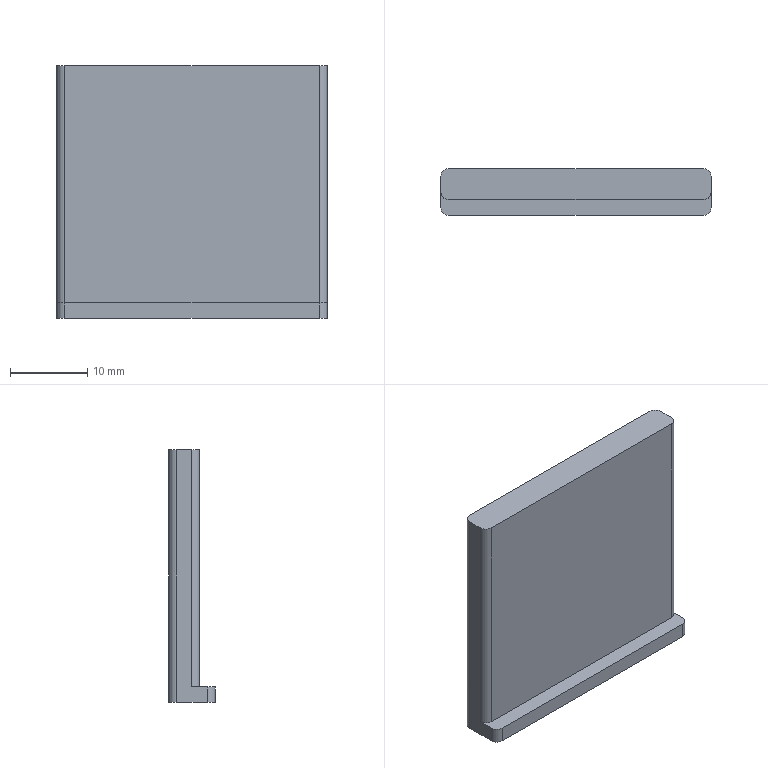Part | STEP file | 1 solid | 14 faces | box 34.97 x 6 x 32.7 mm | volume 4654 mm3 | plane 8 | cylinder 6 | commonest cylinder face diameters 2 x6
STEP:
#1=CARTESIAN_POINT('',(0.,0.,0.));
#2=DIRECTION('',(0.,0.,1.));
#3=DIRECTION('',(1.,0.,0.));
#4=AXIS2_PLACEMENT_3D('',#1,#2,#3);
#5=CARTESIAN_POINT('',(1348.732,487.51,23.619));
#6=VERTEX_POINT('',#5);
#7=CARTESIAN_POINT('',(1315.762,487.51,23.619));
#8=VERTEX_POINT('',#7);
#9=CARTESIAN_POINT('',(1314.747,487.51,23.619));
#10=DIRECTION('',(-1.,0.,0.));
#11=VECTOR('',#10,1.);
#12=LINE('',#9,#11);
#13=CARTESIAN_POINT('',(1314.747,487.51,227.429));
#14=DIRECTION('',(0.,1.,0.));
#15=DIRECTION('',(0.,0.,-1.));
#16=AXIS2_PLACEMENT_3D('',#13,#14,#15);
#17=PLANE('',#16);
#18=CARTESIAN_POINT('',(203.81,0.));
#19=DIRECTION('',(0.,1.));
#20=VECTOR('',#19,1.);
#21=LINE('',#18,#20);
#22=(GEOMETRIC_REPRESENTATION_CONTEXT(2)PARAMETRIC_REPRESENTATION_CONTEXT()REPRESENTATION_CONTEXT('',''));
#23=DEFINITIONAL_REPRESENTATION('',(#21),#22);
#24=PCURVE('',#17,#23);
#25=CARTESIAN_POINT('',(1317.247,584.995,23.619));
#26=DIRECTION('',(0.,0.,-1.));
#27=DIRECTION('',(-1.,0.,0.));
#28=AXIS2_PLACEMENT_3D('',#25,#26,#27);
#29=PLANE('',#28);
#30=CARTESIAN_POINT('',(2.5,-97.485));
#31=DIRECTION('',(1.,0.));
#32=VECTOR('',#31,1.);
#33=LINE('',#30,#32);
#34=(GEOMETRIC_REPRESENTATION_CONTEXT(2)PARAMETRIC_REPRESENTATION_CONTEXT()REPRESENTATION_CONTEXT('',''));
#35=DEFINITIONAL_REPRESENTATION('',(#33),#34);
#36=PCURVE('',#29,#35);
#37=SURFACE_CURVE('',#12,(#24,#36),.PCURVE_S1.);
#38=EDGE_CURVE('',#6,#8,#37,.T.);
#39=ORIENTED_EDGE('',*,*,#38,.T.);
#40=CARTESIAN_POINT('',(1315.762,487.51,-7.081));
#41=VERTEX_POINT('',#40);
#42=CARTESIAN_POINT('',(1315.762,487.51,227.429));
#43=DIRECTION('',(0.,0.,-1.));
#44=VECTOR('',#43,1.);
#45=LINE('',#42,#44);
#46=CARTESIAN_POINT('',(0.,-1.015));
#47=DIRECTION('',(1.,0.));
#48=VECTOR('',#47,1.);
#49=LINE('',#46,#48);
#50=(GEOMETRIC_REPRESENTATION_CONTEXT(2)PARAMETRIC_REPRESENTATION_CONTEXT()REPRESENTATION_CONTEXT('',''));
#51=DEFINITIONAL_REPRESENTATION('',(#49),#50);
#52=PCURVE('',#17,#51);
#53=CARTESIAN_POINT('',(1315.762,488.51,227.429));
#54=DIRECTION('',(0.,0.,-1.));
#55=DIRECTION('',(-1.,0.,0.));
#56=AXIS2_PLACEMENT_3D('',#53,#54,#55);
#57=CYLINDRICAL_SURFACE('',#56,1.);
#58=CARTESIAN_POINT('',(4.712,0.));
#59=DIRECTION('',(0.,1.));
#60=VECTOR('',#59,1.);
#61=LINE('',#58,#60);
#62=(GEOMETRIC_REPRESENTATION_CONTEXT(2)PARAMETRIC_REPRESENTATION_CONTEXT()REPRESENTATION_CONTEXT('',''));
#63=DEFINITIONAL_REPRESENTATION('',(#61),#62);
#64=PCURVE('',#57,#63);
#65=SURFACE_CURVE('',#45,(#52,#64),.PCURVE_S1.);
#66=EDGE_CURVE('',#8,#41,#65,.T.);
#67=ORIENTED_EDGE('',*,*,#66,.T.);
#68=CARTESIAN_POINT('',(1348.732,487.51,-7.081));
#69=VERTEX_POINT('',#68);
#70=CARTESIAN_POINT('',(1349.732,487.51,-7.081));
#71=DIRECTION('',(-1.,0.,0.));
#72=VECTOR('',#71,1.);
#73=LINE('',#70,#72);
#74=CARTESIAN_POINT('',(234.51,-34.985));
#75=DIRECTION('',(0.,1.));
#76=VECTOR('',#75,1.);
#77=LINE('',#74,#76);
#78=(GEOMETRIC_REPRESENTATION_CONTEXT(2)PARAMETRIC_REPRESENTATION_CONTEXT()REPRESENTATION_CONTEXT('',''));
#79=DEFINITIONAL_REPRESENTATION('',(#77),#78);
#80=PCURVE('',#17,#79);
#81=CARTESIAN_POINT('',(1349.732,487.51,-7.081));
#82=DIRECTION('',(0.,0.,1.));
#83=DIRECTION('',(1.,0.,0.));
#84=AXIS2_PLACEMENT_3D('',#81,#82,#83);
#85=PLANE('',#84);
#86=CARTESIAN_POINT('',(0.,0.));
#87=DIRECTION('',(-1.,0.));
#88=VECTOR('',#87,1.);
#89=LINE('',#86,#88);
#90=(GEOMETRIC_REPRESENTATION_CONTEXT(2)PARAMETRIC_REPRESENTATION_CONTEXT()REPRESENTATION_CONTEXT('',''));
#91=DEFINITIONAL_REPRESENTATION('',(#89),#90);
#92=PCURVE('',#85,#91);
#93=SURFACE_CURVE('',#73,(#80,#92),.PCURVE_S1.);
#94=EDGE_CURVE('',#69,#41,#93,.T.);
#95=ORIENTED_EDGE('',*,*,#94,.F.);
#96=CARTESIAN_POINT('',(1348.732,487.51,227.429));
#97=DIRECTION('',(0.,0.,1.));
#98=VECTOR('',#97,1.);
#99=LINE('',#96,#98);
#100=CARTESIAN_POINT('',(0.,-33.985));
#101=DIRECTION('',(-1.,0.));
#102=VECTOR('',#101,1.);
#103=LINE('',#100,#102);
#104=(GEOMETRIC_REPRESENTATION_CONTEXT(2)PARAMETRIC_REPRESENTATION_CONTEXT()REPRESENTATION_CONTEXT('',''));
#105=DEFINITIONAL_REPRESENTATION('',(#103),#104);
#106=PCURVE('',#17,#105);
#107=CARTESIAN_POINT('',(1348.732,488.51,227.429));
#108=DIRECTION('',(0.,0.,-1.));
#109=DIRECTION('',(-1.,0.,0.));
#110=AXIS2_PLACEMENT_3D('',#107,#108,#109);
#111=CYLINDRICAL_SURFACE('',#110,1.);
#112=CARTESIAN_POINT('',(4.712,0.));
#113=DIRECTION('',(0.,-1.));
#114=VECTOR('',#113,1.);
#115=LINE('',#112,#114);
#116=(GEOMETRIC_REPRESENTATION_CONTEXT(2)PARAMETRIC_REPRESENTATION_CONTEXT()REPRESENTATION_CONTEXT('',''));
#117=DEFINITIONAL_REPRESENTATION('',(#115),#116);
#118=PCURVE('',#111,#117);
#119=SURFACE_CURVE('',#99,(#106,#118),.PCURVE_S1.);
#120=EDGE_CURVE('',#69,#6,#119,.T.);
#121=ORIENTED_EDGE('',*,*,#120,.T.);
#122=EDGE_LOOP('',(#39,#67,#95,#121));
#123=FACE_BOUND('',#122,.T.);
#124=ADVANCED_FACE('',(#123),#17,.F.);
#125=CARTESIAN_POINT('',(1314.762,488.51,23.619));
#126=VERTEX_POINT('',#125);
#127=CARTESIAN_POINT('',(1314.762,490.48,23.619));
#128=VERTEX_POINT('',#127);
#129=CARTESIAN_POINT('',(1314.762,491.495,23.619));
#130=DIRECTION('',(0.,1.,0.));
#131=VECTOR('',#130,1.);
#132=LINE('',#129,#131);
#133=CARTESIAN_POINT('',(2.485,-93.5));
#134=DIRECTION('',(0.,1.));
#135=VECTOR('',#134,1.);
#136=LINE('',#133,#135);
#137=(GEOMETRIC_REPRESENTATION_CONTEXT(2)PARAMETRIC_REPRESENTATION_CONTEXT()REPRESENTATION_CONTEXT('',''));
#138=DEFINITIONAL_REPRESENTATION('',(#136),#137);
#139=PCURVE('',#29,#138);
#140=CARTESIAN_POINT('',(1314.762,491.495,227.429));
#141=DIRECTION('',(1.,0.,0.));
#142=DIRECTION('',(0.,0.,-1.));
#143=AXIS2_PLACEMENT_3D('',#140,#141,#142);
#144=PLANE('',#143);
#145=CARTESIAN_POINT('',(203.81,0.));
#146=DIRECTION('',(0.,1.));
#147=VECTOR('',#146,1.);
#148=LINE('',#145,#147);
#149=(GEOMETRIC_REPRESENTATION_CONTEXT(2)PARAMETRIC_REPRESENTATION_CONTEXT()REPRESENTATION_CONTEXT('',''));
#150=DEFINITIONAL_REPRESENTATION('',(#148),#149);
#151=PCURVE('',#144,#150);
#152=SURFACE_CURVE('',#132,(#139,#151),.PCURVE_S1.);
#153=EDGE_CURVE('',#126,#128,#152,.T.);
#154=ORIENTED_EDGE('',*,*,#153,.F.);
#155=CARTESIAN_POINT('',(1315.762,488.51,23.619));
#156=DIRECTION('',(0.,0.,1.));
#157=DIRECTION('',(1.,0.,0.));
#158=AXIS2_PLACEMENT_3D('',#155,#156,#157);
#159=CIRCLE('',#158,1.);
#160=CARTESIAN_POINT('',(0.4851,-96.485));
#161=CARTESIAN_POINT('',(0.4851,-94.753));
#162=CARTESIAN_POINT('',(1.985,-95.619));
#163=CARTESIAN_POINT('',(3.485,-96.485));
#164=CARTESIAN_POINT('',(1.985,-97.351));
#165=CARTESIAN_POINT('',(0.4851,-98.217));
#166=CARTESIAN_POINT('',(0.4851,-96.485));
#167=(BOUNDED_CURVE()B_SPLINE_CURVE(2,(#160,#161,#162,#163,#164,#165,#166),.UNSPECIFIED.,.T.,.F.)B_SPLINE_CURVE_WITH_KNOTS((1,2,2,2,2,1),(-2.094,0.,2.094,4.189,6.283,8.378),.UNSPECIFIED.)CURVE()GEOMETRIC_REPRESENTATION_ITEM()RATIONAL_B_SPLINE_CURVE((1.,0.5,1.,0.5,1.,0.5,1.))REPRESENTATION_ITEM(''));
#168=(GEOMETRIC_REPRESENTATION_CONTEXT(2)PARAMETRIC_REPRESENTATION_CONTEXT()REPRESENTATION_CONTEXT('',''));
#169=DEFINITIONAL_REPRESENTATION('',(#167),#168);
#170=PCURVE('',#29,#169);
#171=CARTESIAN_POINT('',(9.425,203.81));
#172=DIRECTION('',(-1.,0.));
#173=VECTOR('',#172,1.);
#174=LINE('',#171,#173);
#175=(GEOMETRIC_REPRESENTATION_CONTEXT(2)PARAMETRIC_REPRESENTATION_CONTEXT()REPRESENTATION_CONTEXT('',''));
#176=DEFINITIONAL_REPRESENTATION('',(#174),#175);
#177=PCURVE('',#57,#176);
#178=SURFACE_CURVE('',#159,(#170,#177),.PCURVE_S1.);
#179=EDGE_CURVE('',#126,#8,#178,.T.);
#180=ORIENTED_EDGE('',*,*,#179,.T.);
#181=ORIENTED_EDGE('',*,*,#38,.F.);
#182=CARTESIAN_POINT('',(1349.732,488.51,23.619));
#183=VERTEX_POINT('',#182);
#184=CARTESIAN_POINT('',(1348.732,488.51,23.619));
#185=DIRECTION('',(0.,0.,1.));
#186=DIRECTION('',(1.,0.,0.));
#187=AXIS2_PLACEMENT_3D('',#184,#185,#186);
#188=CIRCLE('',#187,1.);
#189=CARTESIAN_POINT('',(-32.485,-96.485));
#190=CARTESIAN_POINT('',(-32.485,-94.753));
#191=CARTESIAN_POINT('',(-30.985,-95.619));
#192=CARTESIAN_POINT('',(-29.485,-96.485));
#193=CARTESIAN_POINT('',(-30.985,-97.351));
#194=CARTESIAN_POINT('',(-32.485,-98.217));
#195=CARTESIAN_POINT('',(-32.485,-96.485));
#196=(BOUNDED_CURVE()B_SPLINE_CURVE(2,(#189,#190,#191,#192,#193,#194,#195),.UNSPECIFIED.,.T.,.F.)B_SPLINE_CURVE_WITH_KNOTS((1,2,2,2,2,1),(-2.094,0.,2.094,4.189,6.283,8.378),.UNSPECIFIED.)CURVE()GEOMETRIC_REPRESENTATION_ITEM()RATIONAL_B_SPLINE_CURVE((1.,0.5,1.,0.5,1.,0.5,1.))REPRESENTATION_ITEM(''));
#197=(GEOMETRIC_REPRESENTATION_CONTEXT(2)PARAMETRIC_REPRESENTATION_CONTEXT()REPRESENTATION_CONTEXT('',''));
#198=DEFINITIONAL_REPRESENTATION('',(#196),#197);
#199=PCURVE('',#29,#198);
#200=CARTESIAN_POINT('',(9.425,203.81));
#201=DIRECTION('',(-1.,0.));
#202=VECTOR('',#201,1.);
#203=LINE('',#200,#202);
#204=(GEOMETRIC_REPRESENTATION_CONTEXT(2)PARAMETRIC_REPRESENTATION_CONTEXT()REPRESENTATION_CONTEXT('',''));
#205=DEFINITIONAL_REPRESENTATION('',(#203),#204);
#206=PCURVE('',#111,#205);
#207=SURFACE_CURVE('',#188,(#199,#206),.PCURVE_S1.);
#208=EDGE_CURVE('',#6,#183,#207,.T.);
#209=ORIENTED_EDGE('',*,*,#208,.T.);
#210=CARTESIAN_POINT('',(1349.732,490.48,23.619));
#211=VERTEX_POINT('',#210);
#212=CARTESIAN_POINT('',(1349.732,487.495,23.619));
#213=DIRECTION('',(0.,-1.,0.));
#214=VECTOR('',#213,1.);
#215=LINE('',#212,#214);
#216=CARTESIAN_POINT('',(-32.485,-97.5));
#217=DIRECTION('',(0.,-1.));
#218=VECTOR('',#217,1.);
#219=LINE('',#216,#218);
#220=(GEOMETRIC_REPRESENTATION_CONTEXT(2)PARAMETRIC_REPRESENTATION_CONTEXT()REPRESENTATION_CONTEXT('',''));
#221=DEFINITIONAL_REPRESENTATION('',(#219),#220);
#222=PCURVE('',#29,#221);
#223=CARTESIAN_POINT('',(1349.732,487.495,227.429));
#224=DIRECTION('',(-1.,0.,0.));
#225=DIRECTION('',(0.,0.,1.));
#226=AXIS2_PLACEMENT_3D('',#223,#224,#225);
#227=PLANE('',#226);
#228=CARTESIAN_POINT('',(-203.81,0.));
#229=DIRECTION('',(0.,-1.));
#230=VECTOR('',#229,1.);
#231=LINE('',#228,#230);
#232=(GEOMETRIC_REPRESENTATION_CONTEXT(2)PARAMETRIC_REPRESENTATION_CONTEXT()REPRESENTATION_CONTEXT('',''));
#233=DEFINITIONAL_REPRESENTATION('',(#231),#232);
#234=PCURVE('',#227,#233);
#235=SURFACE_CURVE('',#215,(#222,#234),.PCURVE_S1.);
#236=EDGE_CURVE('',#211,#183,#235,.T.);
#237=ORIENTED_EDGE('',*,*,#236,.F.);
#238=CARTESIAN_POINT('',(1348.732,491.48,23.619));
#239=VERTEX_POINT('',#238);
#240=CARTESIAN_POINT('',(1348.732,490.48,23.619));
#241=DIRECTION('',(0.,0.,1.));
#242=DIRECTION('',(1.,0.,0.));
#243=AXIS2_PLACEMENT_3D('',#240,#241,#242);
#244=CIRCLE('',#243,1.);
#245=CARTESIAN_POINT('',(-32.485,-94.515));
#246=CARTESIAN_POINT('',(-32.485,-92.783));
#247=CARTESIAN_POINT('',(-30.985,-93.649));
#248=CARTESIAN_POINT('',(-29.485,-94.515));
#249=CARTESIAN_POINT('',(-30.985,-95.381));
#250=CARTESIAN_POINT('',(-32.485,-96.247));
#251=CARTESIAN_POINT('',(-32.485,-94.515));
#252=(BOUNDED_CURVE()B_SPLINE_CURVE(2,(#245,#246,#247,#248,#249,#250,#251),.UNSPECIFIED.,.T.,.F.)B_SPLINE_CURVE_WITH_KNOTS((1,2,2,2,2,1),(-2.094,0.,2.094,4.189,6.283,8.378),.UNSPECIFIED.)CURVE()GEOMETRIC_REPRESENTATION_ITEM()RATIONAL_B_SPLINE_CURVE((1.,0.5,1.,0.5,1.,0.5,1.))REPRESENTATION_ITEM(''));
#253=(GEOMETRIC_REPRESENTATION_CONTEXT(2)PARAMETRIC_REPRESENTATION_CONTEXT()REPRESENTATION_CONTEXT('',''));
#254=DEFINITIONAL_REPRESENTATION('',(#252),#253);
#255=PCURVE('',#29,#254);
#256=CARTESIAN_POINT('',(1348.732,490.48,227.429));
#257=DIRECTION('',(0.,0.,-1.));
#258=DIRECTION('',(-1.,0.,0.));
#259=AXIS2_PLACEMENT_3D('',#256,#257,#258);
#260=CYLINDRICAL_SURFACE('',#259,1.);
#261=CARTESIAN_POINT('',(3.142,203.81));
#262=DIRECTION('',(-1.,0.));
#263=VECTOR('',#262,1.);
#264=LINE('',#261,#263);
#265=(GEOMETRIC_REPRESENTATION_CONTEXT(2)PARAMETRIC_REPRESENTATION_CONTEXT()REPRESENTATION_CONTEXT('',''));
#266=DEFINITIONAL_REPRESENTATION('',(#264),#265);
#267=PCURVE('',#260,#266);
#268=SURFACE_CURVE('',#244,(#255,#267),.PCURVE_S1.);
#269=EDGE_CURVE('',#211,#239,#268,.T.);
#270=ORIENTED_EDGE('',*,*,#269,.T.);
#271=CARTESIAN_POINT('',(1315.762,491.48,23.619));
#272=VERTEX_POINT('',#271);
#273=CARTESIAN_POINT('',(1349.747,491.48,23.619));
#274=DIRECTION('',(1.,0.,0.));
#275=VECTOR('',#274,1.);
#276=LINE('',#273,#275);
#277=CARTESIAN_POINT('',(-32.5,-93.515));
#278=DIRECTION('',(-1.,0.));
#279=VECTOR('',#278,1.);
#280=LINE('',#277,#279);
#281=(GEOMETRIC_REPRESENTATION_CONTEXT(2)PARAMETRIC_REPRESENTATION_CONTEXT()REPRESENTATION_CONTEXT('',''));
#282=DEFINITIONAL_REPRESENTATION('',(#280),#281);
#283=PCURVE('',#29,#282);
#284=CARTESIAN_POINT('',(1349.747,491.48,227.429));
#285=DIRECTION('',(0.,-1.,0.));
#286=DIRECTION('',(0.,0.,1.));
#287=AXIS2_PLACEMENT_3D('',#284,#285,#286);
#288=PLANE('',#287);
#289=CARTESIAN_POINT('',(-203.81,0.));
#290=DIRECTION('',(0.,-1.));
#291=VECTOR('',#290,1.);
#292=LINE('',#289,#291);
#293=(GEOMETRIC_REPRESENTATION_CONTEXT(2)PARAMETRIC_REPRESENTATION_CONTEXT()REPRESENTATION_CONTEXT('',''));
#294=DEFINITIONAL_REPRESENTATION('',(#292),#293);
#295=PCURVE('',#288,#294);
#296=SURFACE_CURVE('',#276,(#283,#295),.PCURVE_S1.);
#297=EDGE_CURVE('',#272,#239,#296,.T.);
#298=ORIENTED_EDGE('',*,*,#297,.F.);
#299=CARTESIAN_POINT('',(1315.762,490.48,23.619));
#300=DIRECTION('',(0.,0.,1.));
#301=DIRECTION('',(1.,0.,0.));
#302=AXIS2_PLACEMENT_3D('',#299,#300,#301);
#303=CIRCLE('',#302,1.);
#304=CARTESIAN_POINT('',(0.4851,-94.515));
#305=CARTESIAN_POINT('',(0.4851,-92.783));
#306=CARTESIAN_POINT('',(1.985,-93.649));
#307=CARTESIAN_POINT('',(3.485,-94.515));
#308=CARTESIAN_POINT('',(1.985,-95.381));
#309=CARTESIAN_POINT('',(0.4851,-96.247));
#310=CARTESIAN_POINT('',(0.4851,-94.515));
#311=(BOUNDED_CURVE()B_SPLINE_CURVE(2,(#304,#305,#306,#307,#308,#309,#310),.UNSPECIFIED.,.T.,.F.)B_SPLINE_CURVE_WITH_KNOTS((1,2,2,2,2,1),(-2.094,0.,2.094,4.189,6.283,8.378),.UNSPECIFIED.)CURVE()GEOMETRIC_REPRESENTATION_ITEM()RATIONAL_B_SPLINE_CURVE((1.,0.5,1.,0.5,1.,0.5,1.))REPRESENTATION_ITEM(''));
#312=(GEOMETRIC_REPRESENTATION_CONTEXT(2)PARAMETRIC_REPRESENTATION_CONTEXT()REPRESENTATION_CONTEXT('',''));
#313=DEFINITIONAL_REPRESENTATION('',(#311),#312);
#314=PCURVE('',#29,#313);
#315=CARTESIAN_POINT('',(1315.762,490.48,227.429));
#316=DIRECTION('',(0.,0.,-1.));
#317=DIRECTION('',(-1.,0.,0.));
#318=AXIS2_PLACEMENT_3D('',#315,#316,#317);
#319=CYLINDRICAL_SURFACE('',#318,1.);
#320=CARTESIAN_POINT('',(3.142,203.81));
#321=DIRECTION('',(-1.,0.));
#322=VECTOR('',#321,1.);
#323=LINE('',#320,#322);
#324=(GEOMETRIC_REPRESENTATION_CONTEXT(2)PARAMETRIC_REPRESENTATION_CONTEXT()REPRESENTATION_CONTEXT('',''));
#325=DEFINITIONAL_REPRESENTATION('',(#323),#324);
#326=PCURVE('',#319,#325);
#327=SURFACE_CURVE('',#303,(#314,#326),.PCURVE_S1.);
#328=EDGE_CURVE('',#272,#128,#327,.T.);
#329=ORIENTED_EDGE('',*,*,#328,.T.);
#330=EDGE_LOOP('',(#154,#180,#181,#209,#237,#270,#298,#329));
#331=FACE_BOUND('',#330,.T.);
#332=ADVANCED_FACE('',(#331),#29,.F.);
#333=CARTESIAN_POINT('',(1349.732,490.48,-9.081));
#334=VERTEX_POINT('',#333);
#335=CARTESIAN_POINT('',(1349.732,486.48,-9.081));
#336=VERTEX_POINT('',#335);
#337=CARTESIAN_POINT('',(1349.732,487.495,-9.081));
#338=DIRECTION('',(0.,-1.,0.));
#339=VECTOR('',#338,1.);
#340=LINE('',#337,#339);
#341=CARTESIAN_POINT('',(1355.983,448.495,-9.081));
#342=DIRECTION('',(0.,0.,-1.));
#343=DIRECTION('',(-1.,0.,0.));
#344=AXIS2_PLACEMENT_3D('',#341,#342,#343);
#345=PLANE('',#344);
#346=CARTESIAN_POINT('',(6.251,39.));
#347=DIRECTION('',(0.,-1.));
#348=VECTOR('',#347,1.);
#349=LINE('',#346,#348);
#350=(GEOMETRIC_REPRESENTATION_CONTEXT(2)PARAMETRIC_REPRESENTATION_CONTEXT()REPRESENTATION_CONTEXT('',''));
#351=DEFINITIONAL_REPRESENTATION('',(#349),#350);
#352=PCURVE('',#345,#351);
#353=CARTESIAN_POINT('',(-236.51,0.));
#354=DIRECTION('',(0.,-1.));
#355=VECTOR('',#354,1.);
#356=LINE('',#353,#355);
#357=(GEOMETRIC_REPRESENTATION_CONTEXT(2)PARAMETRIC_REPRESENTATION_CONTEXT()REPRESENTATION_CONTEXT('',''));
#358=DEFINITIONAL_REPRESENTATION('',(#356),#357);
#359=PCURVE('',#227,#358);
#360=SURFACE_CURVE('',#340,(#352,#359),.PCURVE_S1.);
#361=EDGE_CURVE('',#334,#336,#360,.T.);
#362=ORIENTED_EDGE('',*,*,#361,.T.);
#363=CARTESIAN_POINT('',(1348.732,485.48,-9.081));
#364=VERTEX_POINT('',#363);
#365=CARTESIAN_POINT('',(1348.732,486.48,-9.081));
#366=DIRECTION('',(0.,0.,-1.));
#367=DIRECTION('',(1.,0.,0.));
#368=AXIS2_PLACEMENT_3D('',#365,#366,#367);
#369=CIRCLE('',#368,1.);
#370=CARTESIAN_POINT('',(7.251,37.985));
#371=DIRECTION('',(-1.,0.));
#372=AXIS2_PLACEMENT_2D('',#370,#371);
#373=CIRCLE('',#372,1.);
#374=(GEOMETRIC_REPRESENTATION_CONTEXT(2)PARAMETRIC_REPRESENTATION_CONTEXT()REPRESENTATION_CONTEXT('',''));
#375=DEFINITIONAL_REPRESENTATION('',(#373),#374);
#376=PCURVE('',#345,#375);
#377=CARTESIAN_POINT('',(1348.732,486.48,43.619));
#378=DIRECTION('',(0.,0.,-1.));
#379=DIRECTION('',(-1.,0.,0.));
#380=AXIS2_PLACEMENT_3D('',#377,#378,#379);
#381=CYLINDRICAL_SURFACE('',#380,1.);
#382=CARTESIAN_POINT('',(3.142,52.7));
#383=DIRECTION('',(1.,0.));
#384=VECTOR('',#383,1.);
#385=LINE('',#382,#384);
#386=(GEOMETRIC_REPRESENTATION_CONTEXT(2)PARAMETRIC_REPRESENTATION_CONTEXT()REPRESENTATION_CONTEXT('',''));
#387=DEFINITIONAL_REPRESENTATION('',(#385),#386);
#388=PCURVE('',#381,#387);
#389=SURFACE_CURVE('',#369,(#376,#388),.PCURVE_S1.);
#390=EDGE_CURVE('',#336,#364,#389,.T.);
#391=ORIENTED_EDGE('',*,*,#390,.T.);
#392=CARTESIAN_POINT('',(1315.762,485.48,-9.081));
#393=VERTEX_POINT('',#392);
#394=CARTESIAN_POINT('',(1314.762,485.48,-9.081));
#395=DIRECTION('',(1.,0.,0.));
#396=VECTOR('',#395,1.);
#397=LINE('',#394,#396);
#398=CARTESIAN_POINT('',(41.221,36.985));
#399=DIRECTION('',(-1.,0.));
#400=VECTOR('',#399,1.);
#401=LINE('',#398,#400);
#402=(GEOMETRIC_REPRESENTATION_CONTEXT(2)PARAMETRIC_REPRESENTATION_CONTEXT()REPRESENTATION_CONTEXT('',''));
#403=DEFINITIONAL_REPRESENTATION('',(#401),#402);
#404=PCURVE('',#345,#403);
#405=CARTESIAN_POINT('',(18203.395,485.48,43.619));
#406=DIRECTION('',(0.,-1.,0.));
#407=DIRECTION('',(0.,0.,1.));
#408=AXIS2_PLACEMENT_3D('',#405,#406,#407);
#409=PLANE('',#408);
#410=CARTESIAN_POINT('',(-52.7,16888.633));
#411=DIRECTION('',(0.,-1.));
#412=VECTOR('',#411,1.);
#413=LINE('',#410,#412);
#414=(GEOMETRIC_REPRESENTATION_CONTEXT(2)PARAMETRIC_REPRESENTATION_CONTEXT()REPRESENTATION_CONTEXT('',''));
#415=DEFINITIONAL_REPRESENTATION('',(#413),#414);
#416=PCURVE('',#409,#415);
#417=SURFACE_CURVE('',#397,(#404,#416),.PCURVE_S1.);
#418=EDGE_CURVE('',#393,#364,#417,.T.);
#419=ORIENTED_EDGE('',*,*,#418,.F.);
#420=CARTESIAN_POINT('',(1314.762,486.48,-9.081));
#421=VERTEX_POINT('',#420);
#422=CARTESIAN_POINT('',(1315.762,486.48,-9.081));
#423=DIRECTION('',(0.,0.,-1.));
#424=DIRECTION('',(1.,0.,0.));
#425=AXIS2_PLACEMENT_3D('',#422,#423,#424);
#426=CIRCLE('',#425,1.);
#427=CARTESIAN_POINT('',(40.221,37.985));
#428=DIRECTION('',(-1.,0.));
#429=AXIS2_PLACEMENT_2D('',#427,#428);
#430=CIRCLE('',#429,1.);
#431=(GEOMETRIC_REPRESENTATION_CONTEXT(2)PARAMETRIC_REPRESENTATION_CONTEXT()REPRESENTATION_CONTEXT('',''));
#432=DEFINITIONAL_REPRESENTATION('',(#430),#431);
#433=PCURVE('',#345,#432);
#434=CARTESIAN_POINT('',(1315.762,486.48,43.619));
#435=DIRECTION('',(0.,0.,1.));
#436=DIRECTION('',(1.,0.,0.));
#437=AXIS2_PLACEMENT_3D('',#434,#435,#436);
#438=CYLINDRICAL_SURFACE('',#437,1.);
#439=CARTESIAN_POINT('',(6.283,-52.7));
#440=DIRECTION('',(-1.,0.));
#441=VECTOR('',#440,1.);
#442=LINE('',#439,#441);
#443=(GEOMETRIC_REPRESENTATION_CONTEXT(2)PARAMETRIC_REPRESENTATION_CONTEXT()REPRESENTATION_CONTEXT('',''));
#444=DEFINITIONAL_REPRESENTATION('',(#442),#443);
#445=PCURVE('',#438,#444);
#446=SURFACE_CURVE('',#426,(#433,#445),.PCURVE_S1.);
#447=EDGE_CURVE('',#393,#421,#446,.T.);
#448=ORIENTED_EDGE('',*,*,#447,.T.);
#449=CARTESIAN_POINT('',(1314.762,490.48,-9.081));
#450=VERTEX_POINT('',#449);
#451=CARTESIAN_POINT('',(1314.762,491.495,-9.081));
#452=DIRECTION('',(0.,1.,0.));
#453=VECTOR('',#452,1.);
#454=LINE('',#451,#453);
#455=CARTESIAN_POINT('',(41.221,43.));
#456=DIRECTION('',(0.,1.));
#457=VECTOR('',#456,1.);
#458=LINE('',#455,#457);
#459=(GEOMETRIC_REPRESENTATION_CONTEXT(2)PARAMETRIC_REPRESENTATION_CONTEXT()REPRESENTATION_CONTEXT('',''));
#460=DEFINITIONAL_REPRESENTATION('',(#458),#459);
#461=PCURVE('',#345,#460);
#462=CARTESIAN_POINT('',(236.51,0.));
#463=DIRECTION('',(0.,1.));
#464=VECTOR('',#463,1.);
#465=LINE('',#462,#464);
#466=(GEOMETRIC_REPRESENTATION_CONTEXT(2)PARAMETRIC_REPRESENTATION_CONTEXT()REPRESENTATION_CONTEXT('',''));
#467=DEFINITIONAL_REPRESENTATION('',(#465),#466);
#468=PCURVE('',#144,#467);
#469=SURFACE_CURVE('',#454,(#461,#468),.PCURVE_S1.);
#470=EDGE_CURVE('',#421,#450,#469,.T.);
#471=ORIENTED_EDGE('',*,*,#470,.T.);
#472=CARTESIAN_POINT('',(1315.762,491.48,-9.081));
#473=VERTEX_POINT('',#472);
#474=CARTESIAN_POINT('',(1315.762,490.48,-9.081));
#475=DIRECTION('',(0.,0.,-1.));
#476=DIRECTION('',(1.,0.,0.));
#477=AXIS2_PLACEMENT_3D('',#474,#475,#476);
#478=CIRCLE('',#477,1.);
#479=CARTESIAN_POINT('',(40.221,41.985));
#480=DIRECTION('',(-1.,0.));
#481=AXIS2_PLACEMENT_2D('',#479,#480);
#482=CIRCLE('',#481,1.);
#483=(GEOMETRIC_REPRESENTATION_CONTEXT(2)PARAMETRIC_REPRESENTATION_CONTEXT()REPRESENTATION_CONTEXT('',''));
#484=DEFINITIONAL_REPRESENTATION('',(#482),#483);
#485=PCURVE('',#345,#484);
#486=CARTESIAN_POINT('',(-3.142,236.51));
#487=DIRECTION('',(1.,0.));
#488=VECTOR('',#487,1.);
#489=LINE('',#486,#488);
#490=(GEOMETRIC_REPRESENTATION_CONTEXT(2)PARAMETRIC_REPRESENTATION_CONTEXT()REPRESENTATION_CONTEXT('',''));
#491=DEFINITIONAL_REPRESENTATION('',(#489),#490);
#492=PCURVE('',#319,#491);
#493=SURFACE_CURVE('',#478,(#485,#492),.PCURVE_S1.);
#494=EDGE_CURVE('',#450,#473,#493,.T.);
#495=ORIENTED_EDGE('',*,*,#494,.T.);
#496=CARTESIAN_POINT('',(1348.732,491.48,-9.081));
#497=VERTEX_POINT('',#496);
#498=CARTESIAN_POINT('',(1349.747,491.48,-9.081));
#499=DIRECTION('',(1.,0.,0.));
#500=VECTOR('',#499,1.);
#501=LINE('',#498,#500);
#502=CARTESIAN_POINT('',(6.236,42.985));
#503=DIRECTION('',(-1.,0.));
#504=VECTOR('',#503,1.);
#505=LINE('',#502,#504);
#506=(GEOMETRIC_REPRESENTATION_CONTEXT(2)PARAMETRIC_REPRESENTATION_CONTEXT()REPRESENTATION_CONTEXT('',''));
#507=DEFINITIONAL_REPRESENTATION('',(#505),#506);
#508=PCURVE('',#345,#507);
#509=CARTESIAN_POINT('',(-236.51,0.));
#510=DIRECTION('',(0.,-1.));
#511=VECTOR('',#510,1.);
#512=LINE('',#509,#511);
#513=(GEOMETRIC_REPRESENTATION_CONTEXT(2)PARAMETRIC_REPRESENTATION_CONTEXT()REPRESENTATION_CONTEXT('',''));
#514=DEFINITIONAL_REPRESENTATION('',(#512),#513);
#515=PCURVE('',#288,#514);
#516=SURFACE_CURVE('',#501,(#508,#515),.PCURVE_S1.);
#517=EDGE_CURVE('',#473,#497,#516,.T.);
#518=ORIENTED_EDGE('',*,*,#517,.T.);
#519=CARTESIAN_POINT('',(1348.732,490.48,-9.081));
#520=DIRECTION('',(0.,0.,-1.));
#521=DIRECTION('',(1.,0.,0.));
#522=AXIS2_PLACEMENT_3D('',#519,#520,#521);
#523=CIRCLE('',#522,1.);
#524=CARTESIAN_POINT('',(7.251,41.985));
#525=DIRECTION('',(-1.,0.));
#526=AXIS2_PLACEMENT_2D('',#524,#525);
#527=CIRCLE('',#526,1.);
#528=(GEOMETRIC_REPRESENTATION_CONTEXT(2)PARAMETRIC_REPRESENTATION_CONTEXT()REPRESENTATION_CONTEXT('',''));
#529=DEFINITIONAL_REPRESENTATION('',(#527),#528);
#530=PCURVE('',#345,#529);
#531=CARTESIAN_POINT('',(-3.142,236.51));
#532=DIRECTION('',(1.,0.));
#533=VECTOR('',#532,1.);
#534=LINE('',#531,#533);
#535=(GEOMETRIC_REPRESENTATION_CONTEXT(2)PARAMETRIC_REPRESENTATION_CONTEXT()REPRESENTATION_CONTEXT('',''));
#536=DEFINITIONAL_REPRESENTATION('',(#534),#535);
#537=PCURVE('',#260,#536);
#538=SURFACE_CURVE('',#523,(#530,#537),.PCURVE_S1.);
#539=EDGE_CURVE('',#497,#334,#538,.T.);
#540=ORIENTED_EDGE('',*,*,#539,.T.);
#541=EDGE_LOOP('',(#362,#391,#419,#448,#471,#495,#518,#540));
#542=FACE_BOUND('',#541,.T.);
#543=ADVANCED_FACE('',(#542),#345,.T.);
#544=CARTESIAN_POINT('',(1349.732,488.51,-7.081));
#545=VERTEX_POINT('',#544);
#546=CARTESIAN_POINT('',(1349.732,486.48,-7.081));
#547=VERTEX_POINT('',#546);
#548=CARTESIAN_POINT('',(1349.732,487.51,-7.081));
#549=DIRECTION('',(0.,-1.,0.));
#550=VECTOR('',#549,1.);
#551=LINE('',#548,#550);
#552=CARTESIAN_POINT('',(-234.51,0.015));
#553=DIRECTION('',(0.,-1.));
#554=VECTOR('',#553,1.);
#555=LINE('',#552,#554);
#556=(GEOMETRIC_REPRESENTATION_CONTEXT(2)PARAMETRIC_REPRESENTATION_CONTEXT()REPRESENTATION_CONTEXT('',''));
#557=DEFINITIONAL_REPRESENTATION('',(#555),#556);
#558=PCURVE('',#227,#557);
#559=CARTESIAN_POINT('',(0.,0.));
#560=DIRECTION('',(0.,-1.));
#561=VECTOR('',#560,1.);
#562=LINE('',#559,#561);
#563=(GEOMETRIC_REPRESENTATION_CONTEXT(2)PARAMETRIC_REPRESENTATION_CONTEXT()REPRESENTATION_CONTEXT('',''));
#564=DEFINITIONAL_REPRESENTATION('',(#562),#563);
#565=PCURVE('',#85,#564);
#566=SURFACE_CURVE('',#551,(#558,#565),.PCURVE_S1.);
#567=EDGE_CURVE('',#545,#547,#566,.T.);
#568=ORIENTED_EDGE('',*,*,#567,.T.);
#569=CARTESIAN_POINT('',(1349.732,486.48,-9.081));
#570=DIRECTION('',(0.,0.,-1.));
#571=VECTOR('',#570,1.);
#572=LINE('',#569,#571);
#573=CARTESIAN_POINT('',(-236.51,-1.015));
#574=DIRECTION('',(-1.,0.));
#575=VECTOR('',#574,1.);
#576=LINE('',#573,#575);
#577=(GEOMETRIC_REPRESENTATION_CONTEXT(2)PARAMETRIC_REPRESENTATION_CONTEXT()REPRESENTATION_CONTEXT('',''));
#578=DEFINITIONAL_REPRESENTATION('',(#576),#577);
#579=PCURVE('',#227,#578);
#580=CARTESIAN_POINT('',(3.142,52.7));
#581=DIRECTION('',(0.,1.));
#582=VECTOR('',#581,1.);
#583=LINE('',#580,#582);
#584=(GEOMETRIC_REPRESENTATION_CONTEXT(2)PARAMETRIC_REPRESENTATION_CONTEXT()REPRESENTATION_CONTEXT('',''));
#585=DEFINITIONAL_REPRESENTATION('',(#583),#584);
#586=PCURVE('',#381,#585);
#587=SURFACE_CURVE('',#572,(#579,#586),.PCURVE_S1.);
#588=EDGE_CURVE('',#547,#336,#587,.T.);
#589=ORIENTED_EDGE('',*,*,#588,.T.);
#590=ORIENTED_EDGE('',*,*,#361,.F.);
#591=CARTESIAN_POINT('',(1349.732,490.48,227.429));
#592=DIRECTION('',(0.,0.,1.));
#593=VECTOR('',#592,1.);
#594=LINE('',#591,#593);
#595=CARTESIAN_POINT('',(0.,2.985));
#596=DIRECTION('',(1.,0.));
#597=VECTOR('',#596,1.);
#598=LINE('',#595,#597);
#599=(GEOMETRIC_REPRESENTATION_CONTEXT(2)PARAMETRIC_REPRESENTATION_CONTEXT()REPRESENTATION_CONTEXT('',''));
#600=DEFINITIONAL_REPRESENTATION('',(#598),#599);
#601=PCURVE('',#227,#600);
#602=CARTESIAN_POINT('',(3.142,0.));
#603=DIRECTION('',(0.,-1.));
#604=VECTOR('',#603,1.);
#605=LINE('',#602,#604);
#606=(GEOMETRIC_REPRESENTATION_CONTEXT(2)PARAMETRIC_REPRESENTATION_CONTEXT()REPRESENTATION_CONTEXT('',''));
#607=DEFINITIONAL_REPRESENTATION('',(#605),#606);
#608=PCURVE('',#260,#607);
#609=SURFACE_CURVE('',#594,(#601,#608),.PCURVE_S1.);
#610=EDGE_CURVE('',#334,#211,#609,.T.);
#611=ORIENTED_EDGE('',*,*,#610,.T.);
#612=ORIENTED_EDGE('',*,*,#236,.T.);
#613=CARTESIAN_POINT('',(1349.732,488.51,227.429));
#614=DIRECTION('',(0.,0.,-1.));
#615=VECTOR('',#614,1.);
#616=LINE('',#613,#615);
#617=CARTESIAN_POINT('',(0.,1.015));
#618=DIRECTION('',(-1.,0.));
#619=VECTOR('',#618,1.);
#620=LINE('',#617,#619);
#621=(GEOMETRIC_REPRESENTATION_CONTEXT(2)PARAMETRIC_REPRESENTATION_CONTEXT()REPRESENTATION_CONTEXT('',''));
#622=DEFINITIONAL_REPRESENTATION('',(#620),#621);
#623=PCURVE('',#227,#622);
#624=CARTESIAN_POINT('',(3.142,0.));
#625=DIRECTION('',(0.,1.));
#626=VECTOR('',#625,1.);
#627=LINE('',#624,#626);
#628=(GEOMETRIC_REPRESENTATION_CONTEXT(2)PARAMETRIC_REPRESENTATION_CONTEXT()REPRESENTATION_CONTEXT('',''));
#629=DEFINITIONAL_REPRESENTATION('',(#627),#628);
#630=PCURVE('',#111,#629);
#631=SURFACE_CURVE('',#616,(#623,#630),.PCURVE_S1.);
#632=EDGE_CURVE('',#183,#545,#631,.T.);
#633=ORIENTED_EDGE('',*,*,#632,.T.);
#634=EDGE_LOOP('',(#568,#589,#590,#611,#612,#633));
#635=FACE_BOUND('',#634,.T.);
#636=ADVANCED_FACE('',(#635),#227,.F.);
#637=ORIENTED_EDGE('',*,*,#470,.F.);
#638=CARTESIAN_POINT('',(1314.762,486.48,-7.081));
#639=VERTEX_POINT('',#638);
#640=CARTESIAN_POINT('',(1314.762,486.48,-7.081));
#641=DIRECTION('',(0.,0.,1.));
#642=VECTOR('',#641,1.);
#643=LINE('',#640,#642);
#644=CARTESIAN_POINT('',(234.51,-5.015));
#645=DIRECTION('',(-1.,0.));
#646=VECTOR('',#645,1.);
#647=LINE('',#644,#646);
#648=(GEOMETRIC_REPRESENTATION_CONTEXT(2)PARAMETRIC_REPRESENTATION_CONTEXT()REPRESENTATION_CONTEXT('',''));
#649=DEFINITIONAL_REPRESENTATION('',(#647),#648);
#650=PCURVE('',#144,#649);
#651=CARTESIAN_POINT('',(3.142,-50.7));
#652=DIRECTION('',(0.,1.));
#653=VECTOR('',#652,1.);
#654=LINE('',#651,#653);
#655=(GEOMETRIC_REPRESENTATION_CONTEXT(2)PARAMETRIC_REPRESENTATION_CONTEXT()REPRESENTATION_CONTEXT('',''));
#656=DEFINITIONAL_REPRESENTATION('',(#654),#655);
#657=PCURVE('',#438,#656);
#658=SURFACE_CURVE('',#643,(#650,#657),.PCURVE_S1.);
#659=EDGE_CURVE('',#421,#639,#658,.T.);
#660=ORIENTED_EDGE('',*,*,#659,.T.);
#661=CARTESIAN_POINT('',(1314.762,488.51,-7.081));
#662=VERTEX_POINT('',#661);
#663=CARTESIAN_POINT('',(1314.762,487.51,-7.081));
#664=DIRECTION('',(0.,-1.,0.));
#665=VECTOR('',#664,1.);
#666=LINE('',#663,#665);
#667=CARTESIAN_POINT('',(234.51,-3.985));
#668=DIRECTION('',(0.,-1.));
#669=VECTOR('',#668,1.);
#670=LINE('',#667,#669);
#671=(GEOMETRIC_REPRESENTATION_CONTEXT(2)PARAMETRIC_REPRESENTATION_CONTEXT()REPRESENTATION_CONTEXT('',''));
#672=DEFINITIONAL_REPRESENTATION('',(#670),#671);
#673=PCURVE('',#144,#672);
#674=CARTESIAN_POINT('',(-34.97,0.));
#675=DIRECTION('',(0.,-1.));
#676=VECTOR('',#675,1.);
#677=LINE('',#674,#676);
#678=(GEOMETRIC_REPRESENTATION_CONTEXT(2)PARAMETRIC_REPRESENTATION_CONTEXT()REPRESENTATION_CONTEXT('',''));
#679=DEFINITIONAL_REPRESENTATION('',(#677),#678);
#680=PCURVE('',#85,#679);
#681=SURFACE_CURVE('',#666,(#673,#680),.PCURVE_S1.);
#682=EDGE_CURVE('',#662,#639,#681,.T.);
#683=ORIENTED_EDGE('',*,*,#682,.F.);
#684=CARTESIAN_POINT('',(1314.762,488.51,227.429));
#685=DIRECTION('',(0.,0.,1.));
#686=VECTOR('',#685,1.);
#687=LINE('',#684,#686);
#688=CARTESIAN_POINT('',(0.,-2.985));
#689=DIRECTION('',(-1.,0.));
#690=VECTOR('',#689,1.);
#691=LINE('',#688,#690);
#692=(GEOMETRIC_REPRESENTATION_CONTEXT(2)PARAMETRIC_REPRESENTATION_CONTEXT()REPRESENTATION_CONTEXT('',''));
#693=DEFINITIONAL_REPRESENTATION('',(#691),#692);
#694=PCURVE('',#144,#693);
#695=CARTESIAN_POINT('',(6.283,0.));
#696=DIRECTION('',(0.,-1.));
#697=VECTOR('',#696,1.);
#698=LINE('',#695,#697);
#699=(GEOMETRIC_REPRESENTATION_CONTEXT(2)PARAMETRIC_REPRESENTATION_CONTEXT()REPRESENTATION_CONTEXT('',''));
#700=DEFINITIONAL_REPRESENTATION('',(#698),#699);
#701=PCURVE('',#57,#700);
#702=SURFACE_CURVE('',#687,(#694,#701),.PCURVE_S1.);
#703=EDGE_CURVE('',#662,#126,#702,.T.);
#704=ORIENTED_EDGE('',*,*,#703,.T.);
#705=ORIENTED_EDGE('',*,*,#153,.T.);
#706=CARTESIAN_POINT('',(1314.762,490.48,227.429));
#707=DIRECTION('',(0.,0.,-1.));
#708=VECTOR('',#707,1.);
#709=LINE('',#706,#708);
#710=CARTESIAN_POINT('',(0.,-1.015));
#711=DIRECTION('',(1.,0.));
#712=VECTOR('',#711,1.);
#713=LINE('',#710,#712);
#714=(GEOMETRIC_REPRESENTATION_CONTEXT(2)PARAMETRIC_REPRESENTATION_CONTEXT()REPRESENTATION_CONTEXT('',''));
#715=DEFINITIONAL_REPRESENTATION('',(#713),#714);
#716=PCURVE('',#144,#715);
#717=CARTESIAN_POINT('',(0.,0.));
#718=DIRECTION('',(0.,1.));
#719=VECTOR('',#718,1.);
#720=LINE('',#717,#719);
#721=(GEOMETRIC_REPRESENTATION_CONTEXT(2)PARAMETRIC_REPRESENTATION_CONTEXT()REPRESENTATION_CONTEXT('',''));
#722=DEFINITIONAL_REPRESENTATION('',(#720),#721);
#723=PCURVE('',#319,#722);
#724=SURFACE_CURVE('',#709,(#716,#723),.PCURVE_S1.);
#725=EDGE_CURVE('',#128,#450,#724,.T.);
#726=ORIENTED_EDGE('',*,*,#725,.T.);
#727=EDGE_LOOP('',(#637,#660,#683,#704,#705,#726));
#728=FACE_BOUND('',#727,.T.);
#729=ADVANCED_FACE('',(#728),#144,.F.);
#730=ORIENTED_EDGE('',*,*,#297,.T.);
#731=CARTESIAN_POINT('',(1348.732,491.48,227.429));
#732=DIRECTION('',(0.,0.,-1.));
#733=VECTOR('',#732,1.);
#734=LINE('',#731,#733);
#735=CARTESIAN_POINT('',(0.,1.015));
#736=DIRECTION('',(-1.,0.));
#737=VECTOR('',#736,1.);
#738=LINE('',#735,#737);
#739=(GEOMETRIC_REPRESENTATION_CONTEXT(2)PARAMETRIC_REPRESENTATION_CONTEXT()REPRESENTATION_CONTEXT('',''));
#740=DEFINITIONAL_REPRESENTATION('',(#738),#739);
#741=PCURVE('',#288,#740);
#742=CARTESIAN_POINT('',(1.571,0.));
#743=DIRECTION('',(0.,1.));
#744=VECTOR('',#743,1.);
#745=LINE('',#742,#744);
#746=(GEOMETRIC_REPRESENTATION_CONTEXT(2)PARAMETRIC_REPRESENTATION_CONTEXT()REPRESENTATION_CONTEXT('',''));
#747=DEFINITIONAL_REPRESENTATION('',(#745),#746);
#748=PCURVE('',#260,#747);
#749=SURFACE_CURVE('',#734,(#741,#748),.PCURVE_S1.);
#750=EDGE_CURVE('',#239,#497,#749,.T.);
#751=ORIENTED_EDGE('',*,*,#750,.T.);
#752=ORIENTED_EDGE('',*,*,#517,.F.);
#753=CARTESIAN_POINT('',(1315.762,491.48,227.429));
#754=DIRECTION('',(0.,0.,1.));
#755=VECTOR('',#754,1.);
#756=LINE('',#753,#755);
#757=CARTESIAN_POINT('',(0.,33.985));
#758=DIRECTION('',(1.,0.));
#759=VECTOR('',#758,1.);
#760=LINE('',#757,#759);
#761=(GEOMETRIC_REPRESENTATION_CONTEXT(2)PARAMETRIC_REPRESENTATION_CONTEXT()REPRESENTATION_CONTEXT('',''));
#762=DEFINITIONAL_REPRESENTATION('',(#760),#761);
#763=PCURVE('',#288,#762);
#764=CARTESIAN_POINT('',(1.571,0.));
#765=DIRECTION('',(0.,-1.));
#766=VECTOR('',#765,1.);
#767=LINE('',#764,#766);
#768=(GEOMETRIC_REPRESENTATION_CONTEXT(2)PARAMETRIC_REPRESENTATION_CONTEXT()REPRESENTATION_CONTEXT('',''));
#769=DEFINITIONAL_REPRESENTATION('',(#767),#768);
#770=PCURVE('',#319,#769);
#771=SURFACE_CURVE('',#756,(#763,#770),.PCURVE_S1.);
#772=EDGE_CURVE('',#473,#272,#771,.T.);
#773=ORIENTED_EDGE('',*,*,#772,.T.);
#774=EDGE_LOOP('',(#730,#751,#752,#773));
#775=FACE_BOUND('',#774,.T.);
#776=ADVANCED_FACE('',(#775),#288,.F.);
#777=ORIENTED_EDGE('',*,*,#269,.F.);
#778=ORIENTED_EDGE('',*,*,#610,.F.);
#779=ORIENTED_EDGE('',*,*,#539,.F.);
#780=ORIENTED_EDGE('',*,*,#750,.F.);
#781=EDGE_LOOP('',(#777,#778,#779,#780));
#782=FACE_BOUND('',#781,.T.);
#783=ADVANCED_FACE('',(#782),#260,.T.);
#784=ORIENTED_EDGE('',*,*,#328,.F.);
#785=ORIENTED_EDGE('',*,*,#772,.F.);
#786=ORIENTED_EDGE('',*,*,#494,.F.);
#787=ORIENTED_EDGE('',*,*,#725,.F.);
#788=EDGE_LOOP('',(#784,#785,#786,#787));
#789=FACE_BOUND('',#788,.T.);
#790=ADVANCED_FACE('',(#789),#319,.T.);
#791=CARTESIAN_POINT('',(1348.732,485.48,-7.081));
#792=VERTEX_POINT('',#791);
#793=CARTESIAN_POINT('',(1315.762,485.48,-7.081));
#794=VERTEX_POINT('',#793);
#795=CARTESIAN_POINT('',(1349.732,485.48,-7.081));
#796=DIRECTION('',(-1.,0.,0.));
#797=VECTOR('',#796,1.);
#798=LINE('',#795,#797);
#799=CARTESIAN_POINT('',(0.,-2.03));
#800=DIRECTION('',(-1.,0.));
#801=VECTOR('',#800,1.);
#802=LINE('',#799,#801);
#803=(GEOMETRIC_REPRESENTATION_CONTEXT(2)PARAMETRIC_REPRESENTATION_CONTEXT()REPRESENTATION_CONTEXT('',''));
#804=DEFINITIONAL_REPRESENTATION('',(#802),#803);
#805=PCURVE('',#85,#804);
#806=CARTESIAN_POINT('',(-50.7,16853.663));
#807=DIRECTION('',(0.,1.));
#808=VECTOR('',#807,1.);
#809=LINE('',#806,#808);
#810=(GEOMETRIC_REPRESENTATION_CONTEXT(2)PARAMETRIC_REPRESENTATION_CONTEXT()REPRESENTATION_CONTEXT('',''));
#811=DEFINITIONAL_REPRESENTATION('',(#809),#810);
#812=PCURVE('',#409,#811);
#813=SURFACE_CURVE('',#798,(#805,#812),.PCURVE_S1.);
#814=EDGE_CURVE('',#792,#794,#813,.T.);
#815=ORIENTED_EDGE('',*,*,#814,.F.);
#816=CARTESIAN_POINT('',(1348.732,486.48,-7.081));
#817=DIRECTION('',(0.,0.,1.));
#818=DIRECTION('',(-1.,0.,0.));
#819=AXIS2_PLACEMENT_3D('',#816,#817,#818);
#820=CIRCLE('',#819,1.);
#821=CARTESIAN_POINT('',(-1.,-1.03));
#822=DIRECTION('',(-1.,0.));
#823=AXIS2_PLACEMENT_2D('',#821,#822);
#824=CIRCLE('',#823,1.);
#825=(GEOMETRIC_REPRESENTATION_CONTEXT(2)PARAMETRIC_REPRESENTATION_CONTEXT()REPRESENTATION_CONTEXT('',''));
#826=DEFINITIONAL_REPRESENTATION('',(#824),#825);
#827=PCURVE('',#85,#826);
#828=CARTESIAN_POINT('',(6.283,50.7));
#829=DIRECTION('',(-1.,0.));
#830=VECTOR('',#829,1.);
#831=LINE('',#828,#830);
#832=(GEOMETRIC_REPRESENTATION_CONTEXT(2)PARAMETRIC_REPRESENTATION_CONTEXT()REPRESENTATION_CONTEXT('',''));
#833=DEFINITIONAL_REPRESENTATION('',(#831),#832);
#834=PCURVE('',#381,#833);
#835=SURFACE_CURVE('',#820,(#827,#834),.PCURVE_S1.);
#836=EDGE_CURVE('',#792,#547,#835,.T.);
#837=ORIENTED_EDGE('',*,*,#836,.T.);
#838=ORIENTED_EDGE('',*,*,#567,.F.);
#839=CARTESIAN_POINT('',(1348.732,488.51,-7.081));
#840=DIRECTION('',(0.,0.,-1.));
#841=DIRECTION('',(-1.,0.,0.));
#842=AXIS2_PLACEMENT_3D('',#839,#840,#841);
#843=CIRCLE('',#842,1.);
#844=CARTESIAN_POINT('',(-2.,1.));
#845=CARTESIAN_POINT('',(-2.,2.732));
#846=CARTESIAN_POINT('',(-0.5,1.866));
#847=CARTESIAN_POINT('',(1.,1.));
#848=CARTESIAN_POINT('',(-0.5,0.134));
#849=CARTESIAN_POINT('',(-2.,-0.7321));
#850=CARTESIAN_POINT('',(-2.,1.));
#851=(BOUNDED_CURVE()B_SPLINE_CURVE(2,(#844,#845,#846,#847,#848,#849,#850),.UNSPECIFIED.,.T.,.F.)B_SPLINE_CURVE_WITH_KNOTS((1,2,2,2,2,1),(-2.094,0.,2.094,4.189,6.283,8.378),.UNSPECIFIED.)CURVE()GEOMETRIC_REPRESENTATION_ITEM()RATIONAL_B_SPLINE_CURVE((1.,0.5,1.,0.5,1.,0.5,1.))REPRESENTATION_ITEM(''));
#852=(GEOMETRIC_REPRESENTATION_CONTEXT(2)PARAMETRIC_REPRESENTATION_CONTEXT()REPRESENTATION_CONTEXT('',''));
#853=DEFINITIONAL_REPRESENTATION('',(#851),#852);
#854=PCURVE('',#85,#853);
#855=CARTESIAN_POINT('',(0.,234.51));
#856=DIRECTION('',(1.,0.));
#857=VECTOR('',#856,1.);
#858=LINE('',#855,#857);
#859=(GEOMETRIC_REPRESENTATION_CONTEXT(2)PARAMETRIC_REPRESENTATION_CONTEXT()REPRESENTATION_CONTEXT('',''));
#860=DEFINITIONAL_REPRESENTATION('',(#858),#859);
#861=PCURVE('',#111,#860);
#862=SURFACE_CURVE('',#843,(#854,#861),.PCURVE_S1.);
#863=EDGE_CURVE('',#545,#69,#862,.T.);
#864=ORIENTED_EDGE('',*,*,#863,.T.);
#865=ORIENTED_EDGE('',*,*,#94,.T.);
#866=CARTESIAN_POINT('',(1315.762,488.51,-7.081));
#867=DIRECTION('',(0.,0.,-1.));
#868=DIRECTION('',(-1.,0.,0.));
#869=AXIS2_PLACEMENT_3D('',#866,#867,#868);
#870=CIRCLE('',#869,1.);
#871=CARTESIAN_POINT('',(-34.97,1.));
#872=CARTESIAN_POINT('',(-34.97,2.732));
#873=CARTESIAN_POINT('',(-33.47,1.866));
#874=CARTESIAN_POINT('',(-31.97,1.));
#875=CARTESIAN_POINT('',(-33.47,0.134));
#876=CARTESIAN_POINT('',(-34.97,-0.7321));
#877=CARTESIAN_POINT('',(-34.97,1.));
#878=(BOUNDED_CURVE()B_SPLINE_CURVE(2,(#871,#872,#873,#874,#875,#876,#877),.UNSPECIFIED.,.T.,.F.)B_SPLINE_CURVE_WITH_KNOTS((1,2,2,2,2,1),(-2.094,0.,2.094,4.189,6.283,8.378),.UNSPECIFIED.)CURVE()GEOMETRIC_REPRESENTATION_ITEM()RATIONAL_B_SPLINE_CURVE((1.,0.5,1.,0.5,1.,0.5,1.))REPRESENTATION_ITEM(''));
#879=(GEOMETRIC_REPRESENTATION_CONTEXT(2)PARAMETRIC_REPRESENTATION_CONTEXT()REPRESENTATION_CONTEXT('',''));
#880=DEFINITIONAL_REPRESENTATION('',(#878),#879);
#881=PCURVE('',#85,#880);
#882=CARTESIAN_POINT('',(0.,234.51));
#883=DIRECTION('',(1.,0.));
#884=VECTOR('',#883,1.);
#885=LINE('',#882,#884);
#886=(GEOMETRIC_REPRESENTATION_CONTEXT(2)PARAMETRIC_REPRESENTATION_CONTEXT()REPRESENTATION_CONTEXT('',''));
#887=DEFINITIONAL_REPRESENTATION('',(#885),#886);
#888=PCURVE('',#57,#887);
#889=SURFACE_CURVE('',#870,(#881,#888),.PCURVE_S1.);
#890=EDGE_CURVE('',#41,#662,#889,.T.);
#891=ORIENTED_EDGE('',*,*,#890,.T.);
#892=ORIENTED_EDGE('',*,*,#682,.T.);
#893=CARTESIAN_POINT('',(1315.762,486.48,-7.081));
#894=DIRECTION('',(0.,0.,1.));
#895=DIRECTION('',(-1.,0.,0.));
#896=AXIS2_PLACEMENT_3D('',#893,#894,#895);
#897=CIRCLE('',#896,1.);
#898=CARTESIAN_POINT('',(-33.97,-1.03));
#899=DIRECTION('',(-1.,0.));
#900=AXIS2_PLACEMENT_2D('',#898,#899);
#901=CIRCLE('',#900,1.);
#902=(GEOMETRIC_REPRESENTATION_CONTEXT(2)PARAMETRIC_REPRESENTATION_CONTEXT()REPRESENTATION_CONTEXT('',''));
#903=DEFINITIONAL_REPRESENTATION('',(#901),#902);
#904=PCURVE('',#85,#903);
#905=CARTESIAN_POINT('',(3.142,-50.7));
#906=DIRECTION('',(1.,0.));
#907=VECTOR('',#906,1.);
#908=LINE('',#905,#907);
#909=(GEOMETRIC_REPRESENTATION_CONTEXT(2)PARAMETRIC_REPRESENTATION_CONTEXT()REPRESENTATION_CONTEXT('',''));
#910=DEFINITIONAL_REPRESENTATION('',(#908),#909);
#911=PCURVE('',#438,#910);
#912=SURFACE_CURVE('',#897,(#904,#911),.PCURVE_S1.);
#913=EDGE_CURVE('',#639,#794,#912,.T.);
#914=ORIENTED_EDGE('',*,*,#913,.T.);
#915=EDGE_LOOP('',(#815,#837,#838,#864,#865,#891,#892,#914));
#916=FACE_BOUND('',#915,.T.);
#917=ADVANCED_FACE('',(#916),#85,.T.);
#918=ORIENTED_EDGE('',*,*,#418,.T.);
#919=CARTESIAN_POINT('',(1348.732,485.48,-7.081));
#920=DIRECTION('',(0.,0.,1.));
#921=VECTOR('',#920,1.);
#922=LINE('',#919,#921);
#923=CARTESIAN_POINT('',(-50.7,16854.663));
#924=DIRECTION('',(1.,0.));
#925=VECTOR('',#924,1.);
#926=LINE('',#923,#925);
#927=(GEOMETRIC_REPRESENTATION_CONTEXT(2)PARAMETRIC_REPRESENTATION_CONTEXT()REPRESENTATION_CONTEXT('',''));
#928=DEFINITIONAL_REPRESENTATION('',(#926),#927);
#929=PCURVE('',#409,#928);
#930=CARTESIAN_POINT('',(4.712,50.7));
#931=DIRECTION('',(0.,-1.));
#932=VECTOR('',#931,1.);
#933=LINE('',#930,#932);
#934=(GEOMETRIC_REPRESENTATION_CONTEXT(2)PARAMETRIC_REPRESENTATION_CONTEXT()REPRESENTATION_CONTEXT('',''));
#935=DEFINITIONAL_REPRESENTATION('',(#933),#934);
#936=PCURVE('',#381,#935);
#937=SURFACE_CURVE('',#922,(#929,#936),.PCURVE_S1.);
#938=EDGE_CURVE('',#364,#792,#937,.T.);
#939=ORIENTED_EDGE('',*,*,#938,.T.);
#940=ORIENTED_EDGE('',*,*,#814,.T.);
#941=CARTESIAN_POINT('',(1315.762,485.48,-9.081));
#942=DIRECTION('',(0.,0.,-1.));
#943=VECTOR('',#942,1.);
#944=LINE('',#941,#943);
#945=CARTESIAN_POINT('',(-52.7,16887.633));
#946=DIRECTION('',(-1.,0.));
#947=VECTOR('',#946,1.);
#948=LINE('',#945,#947);
#949=(GEOMETRIC_REPRESENTATION_CONTEXT(2)PARAMETRIC_REPRESENTATION_CONTEXT()REPRESENTATION_CONTEXT('',''));
#950=DEFINITIONAL_REPRESENTATION('',(#948),#949);
#951=PCURVE('',#409,#950);
#952=CARTESIAN_POINT('',(4.712,-52.7));
#953=DIRECTION('',(0.,-1.));
#954=VECTOR('',#953,1.);
#955=LINE('',#952,#954);
#956=(GEOMETRIC_REPRESENTATION_CONTEXT(2)PARAMETRIC_REPRESENTATION_CONTEXT()REPRESENTATION_CONTEXT('',''));
#957=DEFINITIONAL_REPRESENTATION('',(#955),#956);
#958=PCURVE('',#438,#957);
#959=SURFACE_CURVE('',#944,(#951,#958),.PCURVE_S1.);
#960=EDGE_CURVE('',#794,#393,#959,.T.);
#961=ORIENTED_EDGE('',*,*,#960,.T.);
#962=EDGE_LOOP('',(#918,#939,#940,#961));
#963=FACE_BOUND('',#962,.T.);
#964=ADVANCED_FACE('',(#963),#409,.T.);
#965=ORIENTED_EDGE('',*,*,#179,.F.);
#966=ORIENTED_EDGE('',*,*,#703,.F.);
#967=ORIENTED_EDGE('',*,*,#890,.F.);
#968=ORIENTED_EDGE('',*,*,#66,.F.);
#969=EDGE_LOOP('',(#965,#966,#967,#968));
#970=FACE_BOUND('',#969,.T.);
#971=ADVANCED_FACE('',(#970),#57,.T.);
#972=ORIENTED_EDGE('',*,*,#208,.F.);
#973=ORIENTED_EDGE('',*,*,#120,.F.);
#974=ORIENTED_EDGE('',*,*,#863,.F.);
#975=ORIENTED_EDGE('',*,*,#632,.F.);
#976=EDGE_LOOP('',(#972,#973,#974,#975));
#977=FACE_BOUND('',#976,.T.);
#978=ADVANCED_FACE('',(#977),#111,.T.);
#979=ORIENTED_EDGE('',*,*,#390,.F.);
#980=ORIENTED_EDGE('',*,*,#588,.F.);
#981=ORIENTED_EDGE('',*,*,#836,.F.);
#982=ORIENTED_EDGE('',*,*,#938,.F.);
#983=EDGE_LOOP('',(#979,#980,#981,#982));
#984=FACE_BOUND('',#983,.T.);
#985=ADVANCED_FACE('',(#984),#381,.T.);
#986=ORIENTED_EDGE('',*,*,#913,.F.);
#987=ORIENTED_EDGE('',*,*,#659,.F.);
#988=ORIENTED_EDGE('',*,*,#447,.F.);
#989=ORIENTED_EDGE('',*,*,#960,.F.);
#990=EDGE_LOOP('',(#986,#987,#988,#989));
#991=FACE_BOUND('',#990,.T.);
#992=ADVANCED_FACE('',(#991),#438,.T.);
#993=CLOSED_SHELL('',(#124,#332,#543,#636,#729,#776,#783,#790,#917,#964,#971,#978,#985,#992));
#994=MANIFOLD_SOLID_BREP('',#993);
#995=(LENGTH_UNIT()NAMED_UNIT(*)SI_UNIT(.MILLI.,.METRE.));
#996=UNCERTAINTY_MEASURE_WITH_UNIT(LENGTH_MEASURE(0.0000001),#995,'','');
#997=(NAMED_UNIT(*)PLANE_ANGLE_UNIT()SI_UNIT($,.RADIAN.));
#998=(NAMED_UNIT(*)SI_UNIT($,.STERADIAN.)SOLID_ANGLE_UNIT());
#999=(GEOMETRIC_REPRESENTATION_CONTEXT(3)GLOBAL_UNCERTAINTY_ASSIGNED_CONTEXT((#996))GLOBAL_UNIT_ASSIGNED_CONTEXT((#995,#997,#998))REPRESENTATION_CONTEXT('',''));
#1000=ADVANCED_BREP_SHAPE_REPRESENTATION('',(#4,#994),#999);